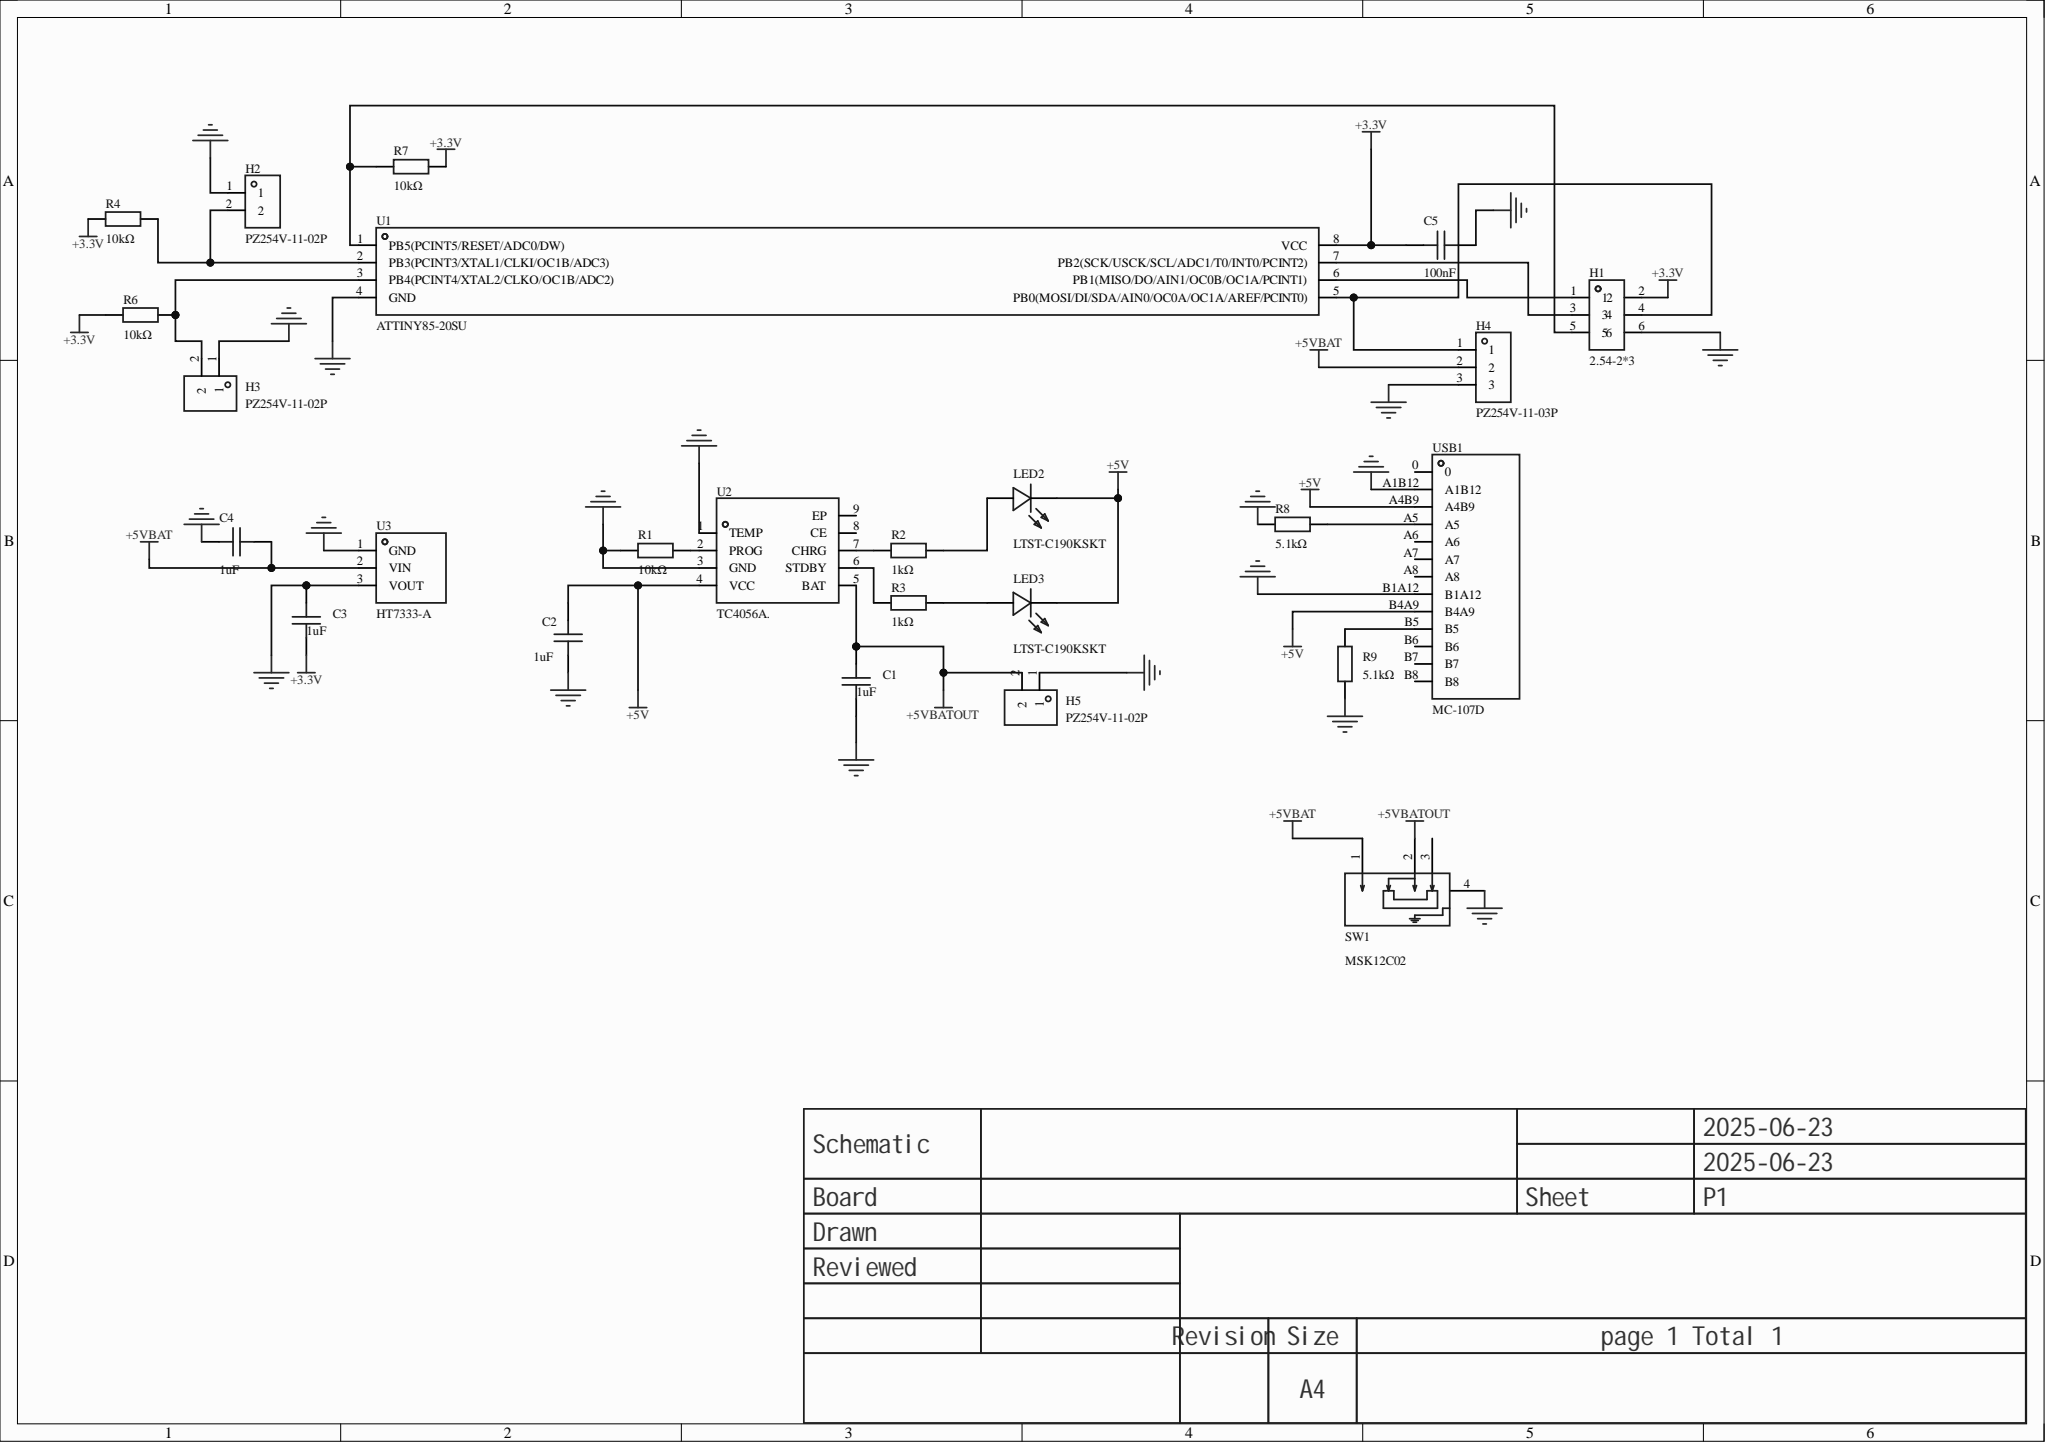Circuit board | Altium Designer | 25 parts | 18 nets
Bill of materials:
Comment,Description,Designator,Footprint,LibRef,Quantity
"1uF","Capacitance: 1uF; tolerance: ±10%; rated voltage: 50V; temperature coefficient: X5R;","C1, C2, C3, C4","C0603","CGA0603X5R105K500JT","4"
"100nF","Capacitance: 1uF; tolerance: ±10%; rated voltage: 50V; temperature coefficient: X5R;","C5","C0603","CGA0603X5R105K500JT","1"
"2.54-2*3","Pin structure: 2x3P; pitch: 2.54mm; rows: double row; total pins: 6P;","H1","HDR-TH_6P-P2.54-V-R2-C3-S2.54_A2541WV-2X3P","2.54-2*3","1"
"PZ254V-11-02P","Pin structure: 1x2P; pitch: 2.54mm; row spacing: -; round/square pin: square pin; mounting: through-hole; rows: single row; total pins: 2P; rated current: -; rated voltage: -; mating pin length: 6mm; plastic height: 2.5mm; tail length: 3mm; contact material: brass; contact plating: -; operating temperature: -40℃~+105℃; color: black;","H2, H3, H5","HDR-TH_2P-P2.54-V-M","PZ254V-11-02P","3"
"PZ254V-11-03P","Pin structure: 1x3P; pitch: 2.54mm; row spacing: -; round/square pin: square pin; mounting: through-hole; rows: single row; total pins: 3P; rated current: 3A; rated voltage: 250V; mating pin length: 6mm; plastic height: 2.5mm; tail length: 3mm; operating temperature: -40℃~+105℃; color: black;","H4","HDR-TH_3P-P2.54-V-M","PZ254V-11-03P","1"
"LTST-C190KSKT","Emitted color: yellow; forward voltage (VF): 2.1V; power: 75mW; forward current: 20mA; dominant wavelength: 584.5nm~597nm; diode configuration: -; lens color: colorless transparent lens; color temperature: -; luminous intensity: 104mcd; viewing angle: 130°; tape and reel: -; operating temperature: -30℃~+85℃;","LED2, LED3","LED0603-RD","LTST-C190KSKT","2"
"10kΩ","Resistor type: thick film resistor; resistance: 10kΩ; tolerance: ±1%; power: 100mW; working voltage: 75V; temperature coefficient: ±100ppm/?;","R1, R4, R6, R7","R0603","0603WAF1002T5E","4"
"1kΩ","Resistor type: thick film resistor; resistance: 10kΩ; tolerance: ±1%; power: 100mW; working voltage: 75V; temperature coefficient: ±100ppm/?;","R2, R3","R0603","0603WAF1002T5E","2"
"5.1kΩ","Resistor type: thick film resistor; resistance: 10kΩ; tolerance: ±1%; power: 100mW; working voltage: 75V; temperature coefficient: ±100ppm/?;","R8, R9","R0603","0603WAF1002T5E","2"
"MSK12C02","Circuit structure: SPDT; mounting: lay-flat SMD; switch color: -; rated current (DC): 50mA; rated voltage (DC): 12V; rated current (AC): -; rated voltage (AC): -; mechanical life: 1万 cycles;","SW1","SW-TH_MSK12C02","MSK12C02","1"
"ATTINY85-20SU","","U1","SOIC-8_L5.3-W5.3-P1.27-LS8.0-BL","ATTINY85-20SU_C31540447","1"
"TC4056A.","","U2","ESOP-8_L4.9-W3.9-P1.27-LS6.0-BL-EP","TC4056A.","1"
"HT7333-A","Output type: fixed; max input voltage: 12V; output voltage: 3.3V; output current: 250mA; power supply rejection ratio (PSRR): -; output polarity: positive;","U3","SOT-89-3_L4.5-W2.5-P1.50-LS4.2-BR","HT7333-A_C347191","1"
"MC-107D","Connector type: Type-C; standard: USB 3.1; gender: female; number of ports: 1; number of contacts: 16P; mounting: lay-flat SMD; rated current - power: 3A; contact material: -; contact plating: -; operating temperature range: -25℃~+85℃; soldering temperature (max): -;","USB1","USB-C-SMD_MC-107D","MC-107D","1"
Netlist (Protel format):
[
C1
C0603
1uF



]
[
C2
C0603
1uF



]
[
C3
C0603
1uF



]
[
C4
C0603
1uF



]
[
C5
C0603
100nF



]
[
H1
HDR-TH_6P-P2.54-V-R2-C3-S2.54_A2541WV-2X3P
2.54-2*3



]
[
H2
HDR-TH_2P-P2.54-V-M
PZ254V-11-02P



]
[
H3
HDR-TH_2P-P2.54-V-M
PZ254V-11-02P



]
[
H4
HDR-TH_3P-P2.54-V-M
PZ254V-11-03P



]
[
H5
HDR-TH_2P-P2.54-V-M
PZ254V-11-02P



]
[
LED2
LED0603-RD
LTST-C190KSKT



]
[
LED3
LED0603-RD
LTST-C190KSKT



]
[
R1
R0603
10kΩ



]
[
R2
R0603
1kΩ



]
[
R3
R0603
1kΩ



]
[
R4
R0603
10kΩ



]
[
R6
R0603
10kΩ



]
[
R7
R0603
10kΩ



]
[
R8
R0603
5.1kΩ



]
[
R9
R0603
5.1kΩ



]
[
SW1
SW-TH_MSK12C02
MSK12C02



]
[
U1
SOIC-8_L5.3-W5.3-P1.27-LS8.0-BL
ATTINY85-20SU



]
[
U2
ESOP-8_L4.9-W3.9-P1.27-LS6.0-BL-EP
TC4056A.



]
[
U3
SOT-89-3_L4.5-W2.5-P1.50-LS4.2-BR
HT7333-A



]
[
USB1
USB-C-SMD_MC-107D
MC-107D



]
(
NetR9_1
R9-1
USB1-B5
)
(
NetR8_2
R8-2
USB1-A5
)
(
NetR3_1
R3-1
U2-6
)
(
NetR2_1
R2-1
U2-7
)
(
NetR1_2
R1-2
U2-2
)
(
NetLED3_2
LED3-2
R3-2
)
(
NetLED2_2
LED2-2
R2-2
)
(
NetH3_2
H3-2
R6-2
U1-3
)
(
NetH2_2
H2-2
R4-1
U1-2
)
(
NetH1_5
H1-5
R7-1
U1-1
)
(
NetH1_4
H1-4
H4-1
U1-5
)
(
NetH1_3
H1-3
U1-7
)
(
NetH1_1
H1-1
U1-6
)
(
GND
C1-1
C2-1
C3-2
C4-2
C5-1
H1-6
H2-1
H3-1
H4-3
H5-1
R1-1
R8-1
R9-2
SW1-4
U1-4
U2-1
U2-3
U3-1
U3-3
USB1-A1B12
USB1-B1A12
)
(
+5VBATOUT
C1-2
H5-2
SW1-2
U2-5
)
(
+5VBAT
C4-1
H4-2
SW1-1
U3-2
)
(
+5V
C2-2
LED2-1
LED3-1
U2-4
USB1-A4B9
USB1-B4A9
)
(
+3.3V
C3-1
C5-2
H1-2
R4-2
R6-1
R7-2
U1-8
)